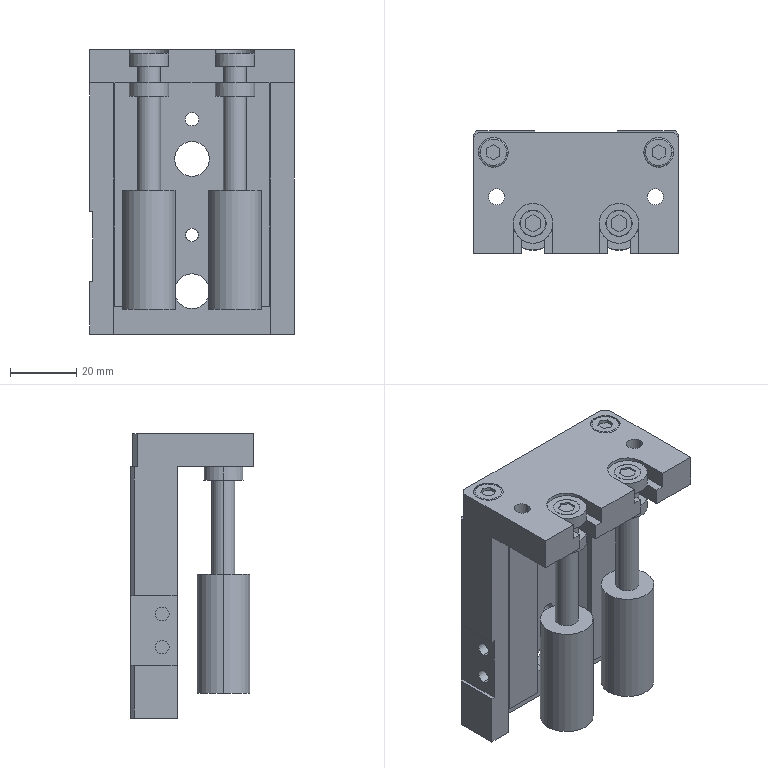Part | SolidWorks | features BaseBody 1, HoleWzd 1, LibraryFeature 1, MoveFace 1 | 1 solid | 176 faces | box 62 x 37 x 86 mm | volume 87128 mm3 | plane 111 | cylinder 61 | spline 4 | commonest cylinder face diameters 4.134 x12 4 x11 12 x8 7 x6 4.917 x4 7.8 x4